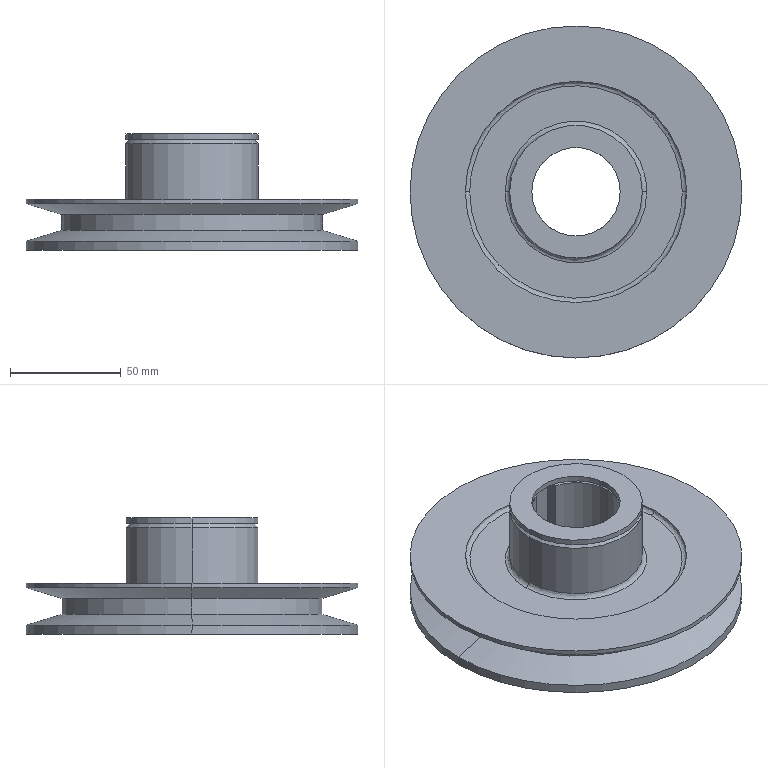Part | SolidWorks | features BaseBody 1 | 1 solid | 44 faces | box 150 x 150 x 52.5 mm | volume 296117 mm3 | cylinder 17 | cone 11 | plane 10 | spline 6 | commonest cylinder face diameters 40 x5 60 x4 150 x4 100 x2 118 x2